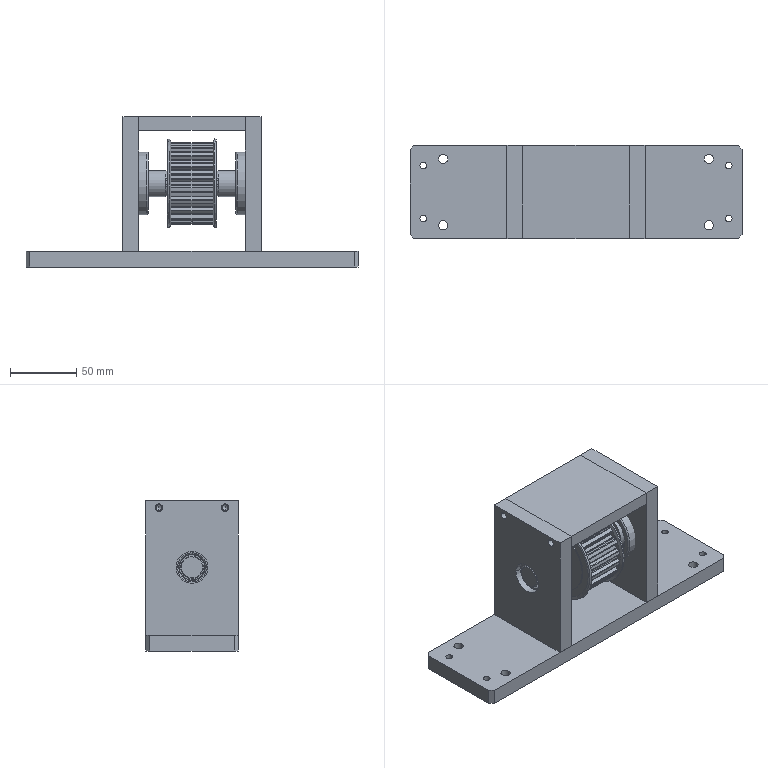Part | SolidWorks | features AEMSimFeature 1, CompositeCurve 1 | 9 solids | 633 faces | box 250 x 70 x 113 mm | volume 559339 mm3 | cylinder 283 | plane 148 | torus 106 | sphere 56 | cone 40 | commonest cylinder face diameters 1 x54 1.2 x50 55.4 x23 61.8 x20 5 x16 7 x16